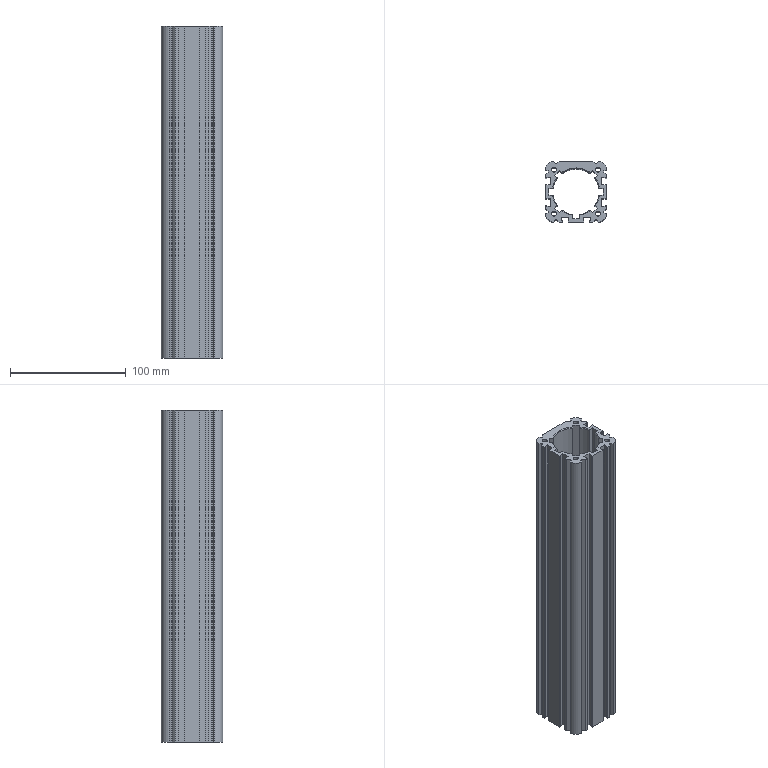Part | STEP file | 03缸体 EDA50-L_R-003-BZ^EDA50-R04 (D60N) | 1 solid | 164 faces | box 53 x 53 x 287 mm | volume 312692 mm3 | plane 99 | cylinder 35 | cone 30 | commonest cylinder face diameters 4.2 x16 4 x8 40 x7 16 x4